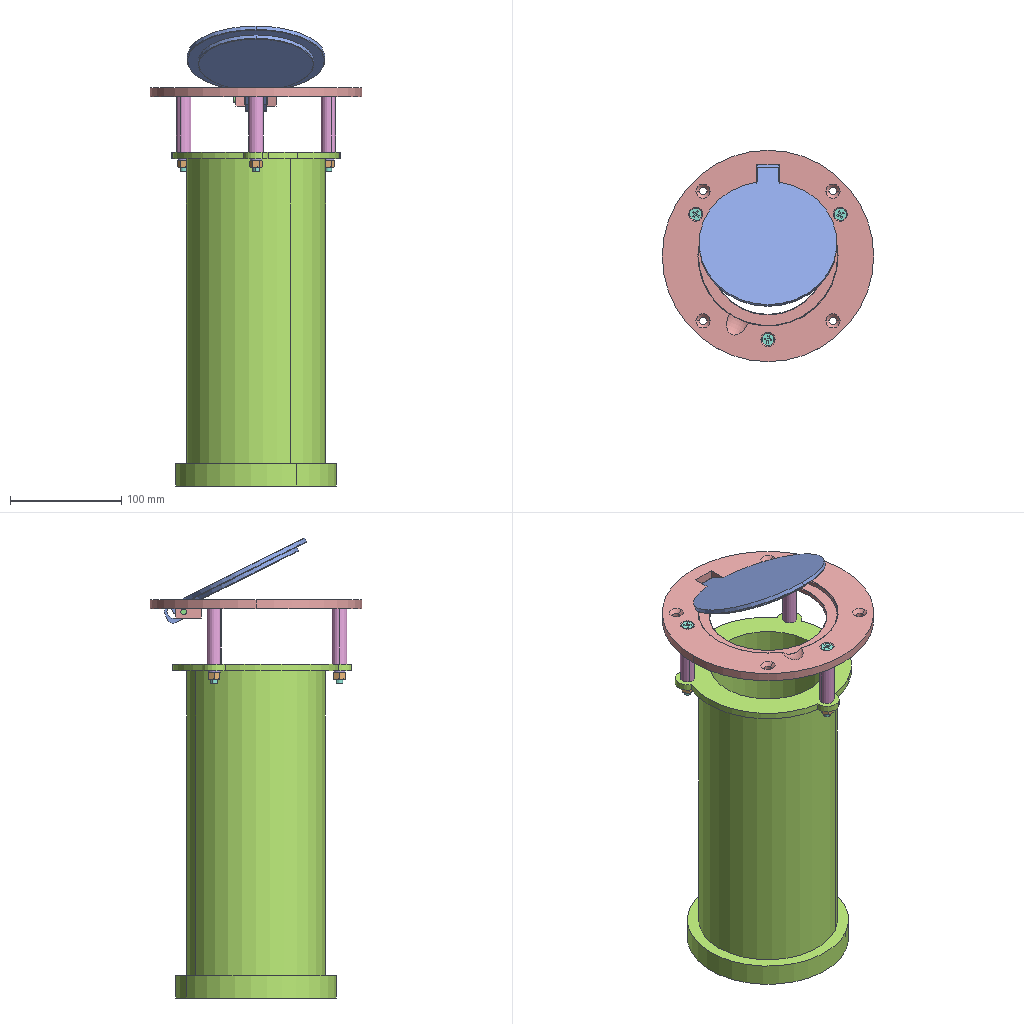Assembly | SolidWorks | 9 different items | 15 placed | box 190 x 190 x 413 mm
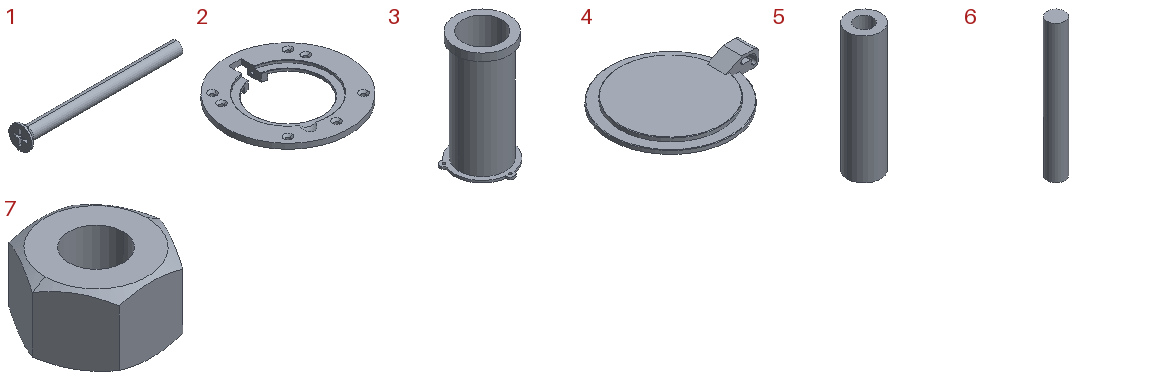Parts list (item | name | quantity | size | volume | features):
1 | - | x3 | 75 x 10.9 x 10.9 mm | 2225 mm3 | features Cut 2, Revolution 2, Draft 1, Fillet 1, LPattern 1, RevCut 1
2 | - | x1 | 190 x 190 x 16.5 mm | 138336 mm3 | features ICE 4, 3DProfileFeature 2, CirPattern 2, HoleWzd 2, Chamfer 1, Extrusion 1, RevCut 1
3 | - | x1 | 151.904 x 161 x 300 mm | 1203905 mm3 | features ICE 2, Extrusion 1
4 | - | x1 | 143 x 124 x 16.5 mm | 87998 mm3 | features ICE 2, Chamfer 1, Extrusion 1, Fillet 1
5 | - | x3 | 13 x 13 x 50 mm | 4712 mm3 | features Extrusion 1
6 | - | x1 | 4.9 x 4.9 x 38 mm | 716.582 mm3 | features Extrusion 1
7 | - | x3 | 11.547 x 10 x 6.4 mm | 424.571 mm3 | features RevCut 2, Extrusion 1, LPattern 1
8 | cross recessed countersunk head screws gb2 | x1 | - | - | -
9 | single coil lock washers light type gb | x1 | - | - | -
Mates (type | each side: item.copy, entity, surface, feature):
Concentric | 2.1 face cylinder Boss-Extrude 1 | 3.1 face cylinder Boss-Extrude 1
Concentric | 2.1 face cylinder CirPattern 1 | 3.1 face cylinder Boss-Extrude 3
DistanceDim | 2.1 face plane Boss-Extrude 1 | 3.1 face plane Boss-Extrude 3
Concentric | 3.1 face cylinder Boss-Extrude 3 | 5.1 face cylinder Boss-Extrude 1
Coincident | 3.1 face plane Boss-Extrude 3 | 5.1 face plane Boss-Extrude 1
Concentric | 5.1 face cylinder Boss-Extrude 1 | 1.1 face cylinder Base
Coincident | 2.1 edge | 1.1 face cone Base
Concentric | 1.1 face cylinder Base | 7.1 face cone Double-Chamfer
DistanceDim | 4.1 face plane Boss-Extrude 3 | 2.1 face plane Cut-Extrude 2
Tangent | 2.1 face cylinder Cut-Extrude 3 | 4.1 face plane Boss-Extrude 3
Concentric | 2.1 face cylinder Cut-Extrude 3 | 4.1 face cylinder Boss-Extrude 3
Concentric | 2.1 face cylinder Cut-Extrude 3 | 6.1 face cylinder Boss-Extrude 1
Coincident | 2.1 face plane Boss-Extrude 2 | 6.1 face plane Boss-Extrude 1